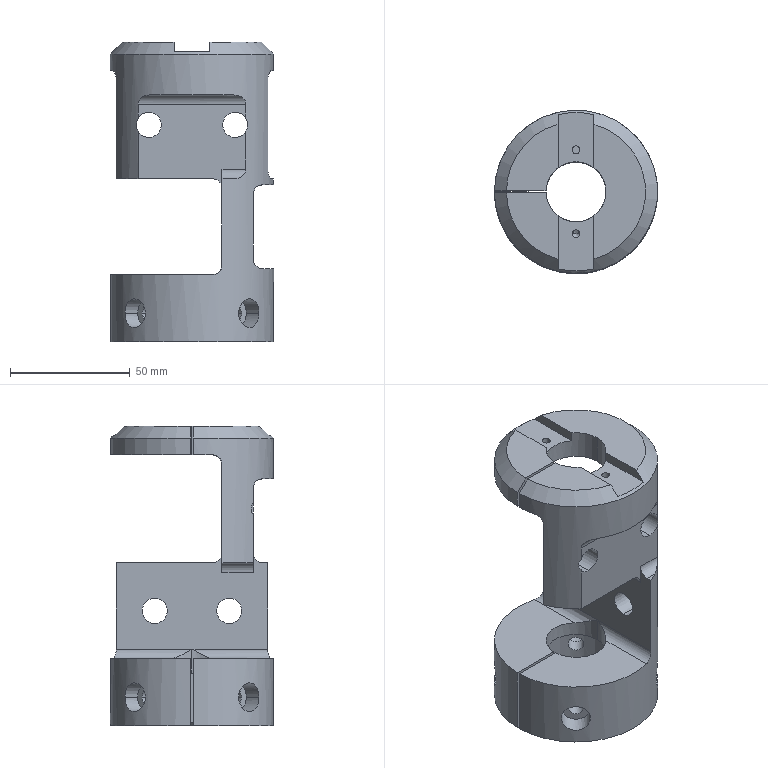Part | SolidWorks | features ICE 17, Fillet 8, MoveFace 7, HoleWzd 3, Chamfer 2, DelFace 1, Extrusion 1, MirrorPattern 1 | 1 solid | 81 faces | box 67.996 x 68 x 125 mm | volume 160312 mm3 | cylinder 44 | plane 33 | cone 4 | commonest cylinder face diameters 8 x10 6.5 x8 10.5 x8 12 x8 3.3 x4 25 x4